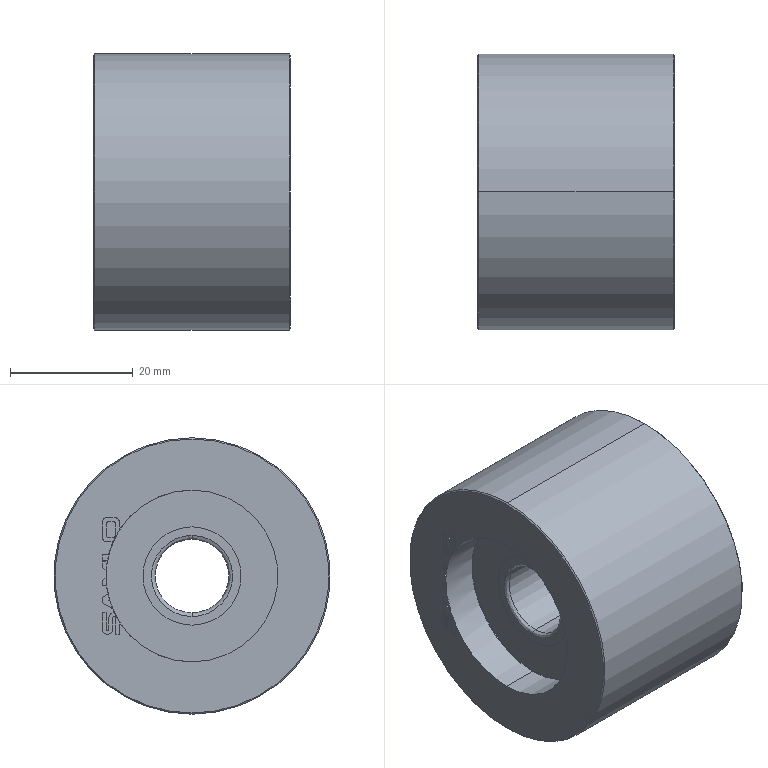Part | SolidWorks | features BaseBody 4 | 4 solids | 141 faces | box 32 x 45 x 45 mm | volume 40105 mm3 | cylinder 62 | plane 59 | spline 16 | cone 4 | commonest cylinder face diameters 28 x10 16 x8 32 x8 0.643 x4 2.5 x4 12 x4